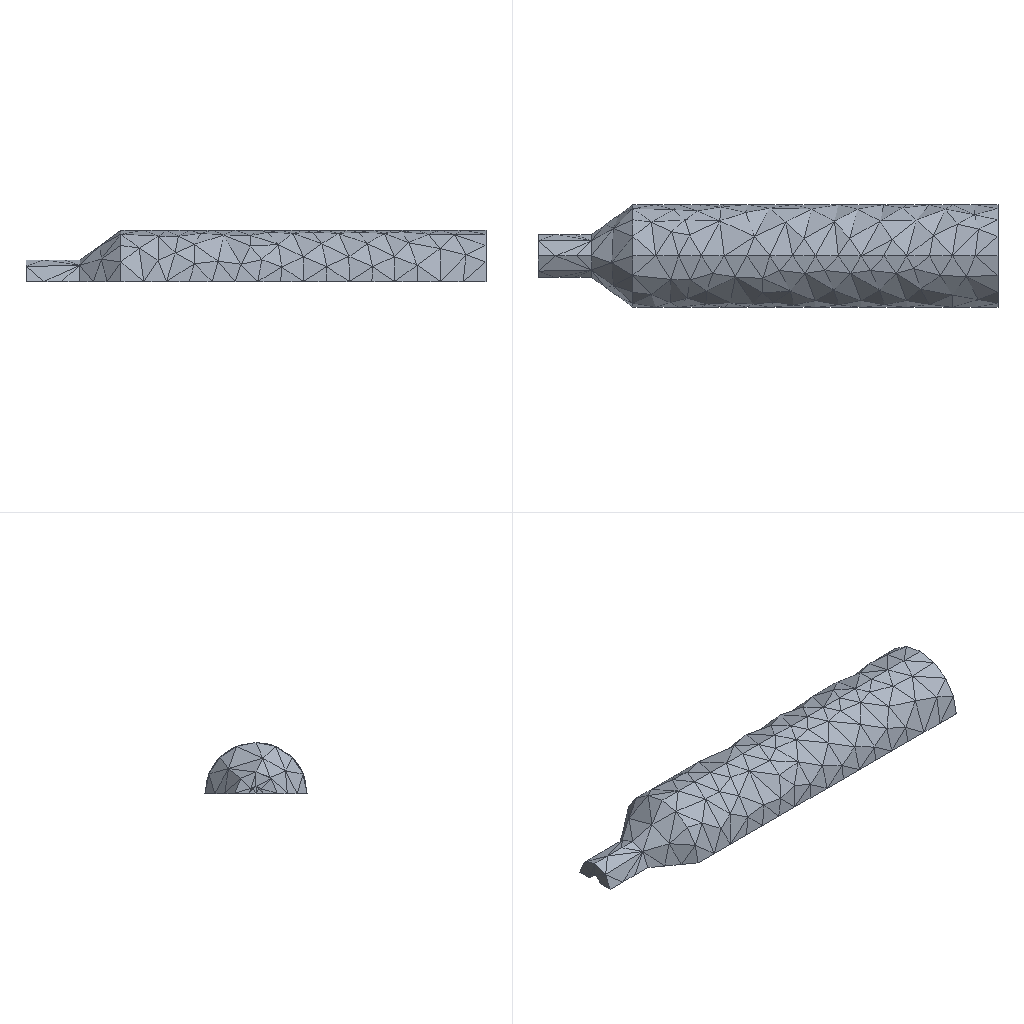Simulation study | ansys workbench
Ansys APDL input file, long lists of numbers shortened:
/batch
/config,noeldb,1     ! force off writing results to database
*get,_wallstrt,active,,time,wall
! ANSYS input file written by Workbench version 2022 R1
! File used for geometry attach:
/title,wbnew--____ (B5)
! ****** Begin Custom Load Command Snippet ******
/COM, ACT Extensions:
/COM,     LSDYNA, 2021.1
/COM,
! ****** End   Custom Load Command Snippet ******
*DIM,_wb_ProjectScratch_dir,string,248
_wb_ProjectScratch_dir(1) = ''
*DIM,_wb_SolverFiles_dir,string,248
_wb_SolverFiles_dir(1) = ''
*DIM,_wb_userfiles_dir,string,248
_wb_userfiles_dir(1) = ''
/com,--- Data in consistent NMM units. See Solving Units in the help system for more information.
/units,MPA
/nopr
/wb,file,start              !  signify a WB generated input file
/prep7
! Turn off shape checking because checks already performed inside WB mesher.
! See help system for more information.
SHPP,OFF,,NOWARN
/nolist
etcon,set             ! allow ANSYS to choose best KEYOP's for 180x elements, resets any applicable keyopt to MAPDL defaults
/com,*********** Nodes for the whole assembly ***********
nblock,3,,1722
(1i9,3e20.9e3)
        1     1.251000000E+03     0.000000000E+00     1.043258926E+02
! (1565 more lines like these left out)
-1
/wb,elem,start            !  set before creation of elements
/com,*********** Elements for Body 1 "__2-FreeParts|__-__4" ***********
et,1,187
eblock,19,solid,,706
(19i9)
        1        1        1        1        0        0        0        0       10        0        1      140      141      174      176     1074     1081     1077     1078
! (1411 more lines like these left out)
-1
/wb,elem,end               !  done creating elements
/com,*********** Send User Defined Coordinate System(s) ***********
csys,0
toffst,273.15,  ! Temperature offset from absolute zero
/com,*********** Set Reference Temperature ***********
tref,22.
/wb,mat,start              !  starting to send materials
/com,*********** Send Materials ***********
Temperature = 'TEMP' ! Temperature
MP,DENS,1,7.85e-09,	! tonne mm^-3
MP,ALPX,1,1.2e-05,	! C^-1
MP,C,1,434000000,	! mm^2 s^-2 C^-1
MP,KXX,1,60.5,	! tonne mm s^-3 C^-1
MP,RSVX,1,0.00017,	! ohm mm
MP,EX,1,200000,	! tonne s^-2 mm^-1
MP,NUXY,1,0.3,
MP,MURX,1,10000,
/wb,mat,end                !  done sending materials
!************************* Model Summary ********************
!__2-FreeParts|__-__4,	结构钢,	matid,	1
!************************* End Model Summary ********************
! get the diagonal of the bounding box. Needed later for other things
*get,_xmin,node,,mnloc,x
*get,_ymin,node,,mnloc,y
*get,_zmin,node,,mnloc,z
*get,_xmax,node,,mxloc,x
*get,_ymax,node,,mxloc,y
*get,_zmax,node,,mxloc,z
_ASMDIAG=(_xmax-_xmin)*(_xmax-_xmin)+(_ymax-_ymin)*(_ymax-_ymin)+(_zmax-_zmin)*(_zmax-_zmin)
_ASMDIAG=SQRT(_ASMDIAG)
/wb,contact,start          !  starting to send contact
/wb,contact,end            !  done creating contacts
/golist
/wb,load,start             !  starting to send loads
/com,*********** Fixed Supports ***********
CMBLOCK,_FIXEDSU,NODE,       36
(8i10)
        57        58        59        60        61        97        98        99
       100       101       102       103       104       708       710       712
       714       715       716       717       719       723       724       725
       731       930       931       933       934       935       937       938
       939       942       950       952
cmsel,s,_FIXEDSU
d,all,all
nsel,all
/com,*********** Define Pressure Using Surface Effect Elements "__" ***********
et,2,154
eblock,10,,,200
(15i9)
     1277        2        2        2        0      102      103      202      202      950      953      202      951
! (199 more lines like these left out)
-1
esel,s,type,,2
keyop,2,7,0                ! Use deformed area for application of load
esel,all
/com,*********** Define Pressure Using Surface Effect Elements "__ 2" ***********
et,3,154
eblock,10,,,164
(15i9)
     1477        3        3        3        0      140      141      178      178     1074     1084      178     1079
! (163 more lines like these left out)
-1
esel,s,type,,3
keyop,3,7,0                ! Use deformed area for application of load
esel,all
esel,all
/gst,on,on
fini
*get,_numnode,node,0,count
*get,_numelem,elem,0,count
*get, _MAXELEMNUM, elem, 0, NUM, MAX
*get, _MAXNODENUM, node, 0, NUM, MAX
*get, _MAXELEMTYPE, etyp, 0, NUM, MAX
*get, _MAXREALCONST, real, 0, NUM, MAX
/go
/wb,load,end               !  done creating loads
/com,--- Number of total nodes = %_numnode%
/com,--- Number of contact elements = 364
/com,--- Number of spring elements = 0
/com,--- Number of bearing elements = 0
/com,--- Number of solid elements = 706
/com,--- Number of condensed parts = 0
/com,--- Number of total elements = %_numelem%
*get,_wallbsol,active,,time,wall
/com,****************************************************************************
/com,*************************    SOLUTION       ********************************
/com,****************************************************************************
/solu
antype,0                   ! static analysis
_thickRatio=  0     ! Ratio of thick parts in the model
eqsl,sparse,,,,,1
cntr,print,1               ! print out contact info and also make no initial contact an error
dmpoption,emat,no             ! Don't combine emat file for DANSYS
dmpoption,esav,no             ! Don't combine esav file for DANSYS
nldiag,cont,iter           ! print out contact info each equilibrium iteration
rescontrol,,none                 ! Do not keep any restart files
/com,****************************************************
/com,******************* SOLVE FOR LS 1 OF 1 ****************
esel,s,type,,2
nsle
sf,all,pres,20.
esel,s,type,,3
nsle
sf,all,pres,60.
nsel,all
esel,all
esel,all
/nopr
/gopr
nsub,1,1,1
time,1.
outres,erase
outres,all,none
outres,nsol,all,
outres,rsol,all
outres,eangl,all
outres,etmp,all
outres,veng,all
outres,strs,all,
outres,epel,all,
outres,eppl,all,
outres,cont,all,
! *********** WB SOLVE COMMAND ***********
! check interactive state
*get,ANSINTER_,active,,int
*if,ANSINTER_,ne,0,then
/eof
*endif
solve
/com *************** Write FE CONNECTORS *********
CEWRITE,file,ce,,INTE
/com,****************************************************
/com,*************** FINISHED SOLVE FOR LS 1 *************
*get,_wallasol,active,,time,wall
/nopr
*get,_numnode,node,0,count
*get,_numelem,elem,0,count
*get, _MAXELEMNUM, elem, 0, NUM, MAX
*get, _MAXNODENUM, node, 0, NUM, MAX,,,INTERNAL
*get, _MAXELEMTYPE, etyp, 0, NUM, MAX
*get, _MAXREALCONST, real, 0, NUM, MAX
/gopr
/post1
xmlo,ENCODING,ISO-8859-1
xmlo,parm
/xml,parm,xml
fini
/gopr
*get,_walldone,active,,time,wall
_preptime=(_wallbsol-_wallstrt)*3600
_solvtime=(_wallasol-_wallbsol)*3600
_posttime=(_walldone-_wallasol)*3600
_totaltim=(_walldone-_wallstrt)*3600
*get,_dlbratio,active,0,solu,dlbr
*get,_combtime,active,0,solu,comb
*get,_ssmode,active,0,solu,ssmm
*get,_ndofs,active,0,solu,ndof
*get,_sol_end_time,active,0,set,time
*if,_sol_end_time,eq,1.,then
/fclean				!clean distributed files
*endif
/com,--- Total number of nodes = %_numnode%
/com,--- Total number of elements = %_numelem%
/com,--- Element load balance ratio = %_dlbratio%
/com,--- Time to combine distributed files = %_combtime%
/com,--- Sparse memory mode = %_ssmode%
/com,--- Number of DOF = %_ndofs%
/wb,file,end               ! done with WB generated input